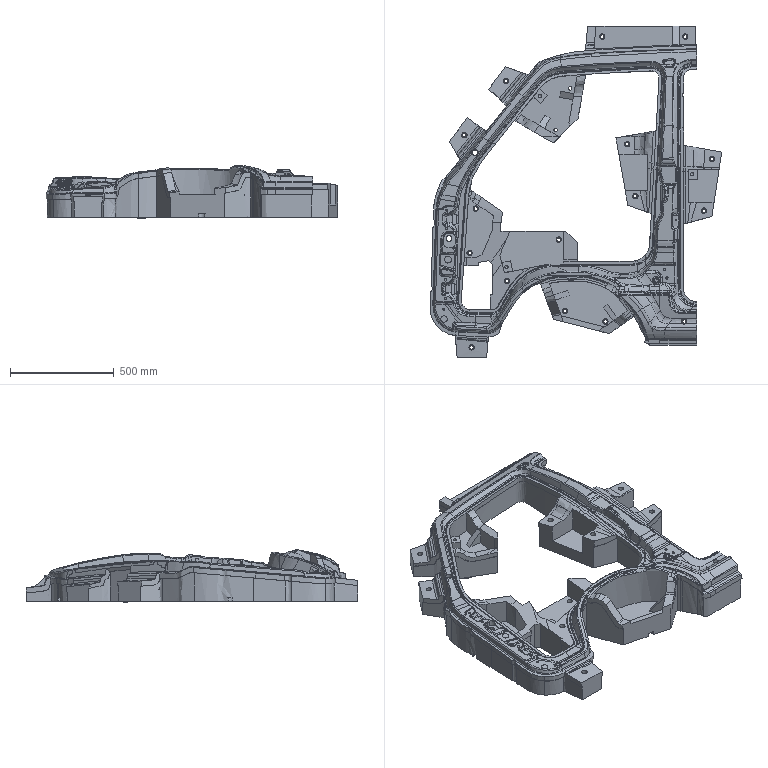Part | NX | features solid 2 | 2 solids | 1527 faces | box 1406 x 1600 x 250.733 mm | volume 138922394 mm3 | spline 1283 | plane 184 | cylinder 57 | cone 3 | commonest cylinder face diameters 17 x18 26 x16 32 x10 40 x4 16 x3 10 x1